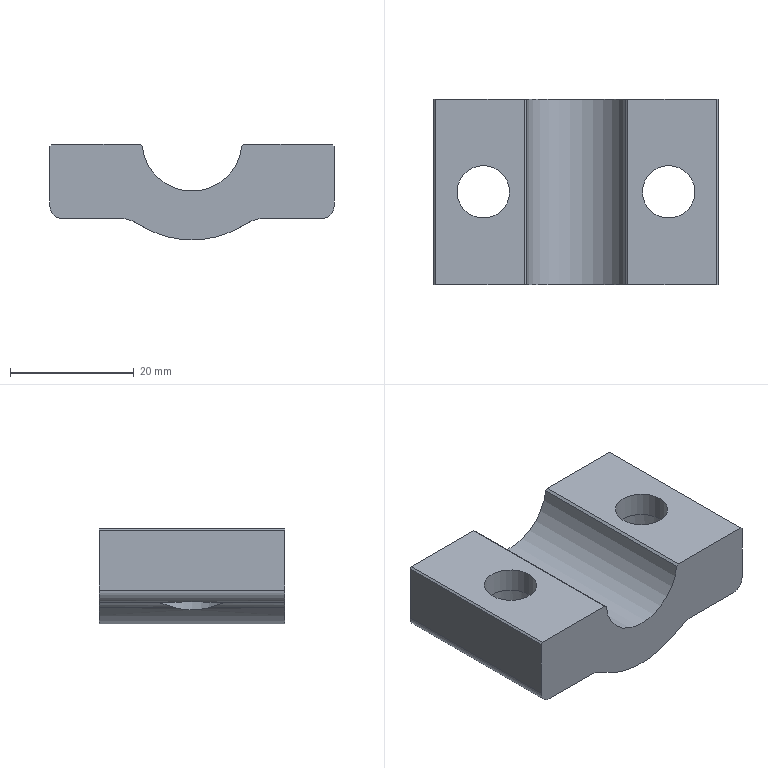NC program | NX | posted with a generic post | part box 46 x 30 x 15.5 mm
Whole program:
N10 G17 G21 G94 G90
(2D点孔 , TOOL : D10点钻)
N12 T04 M6
N14 G54
N16 G17 G0 G90 X-15. Y0. B0. C0. S2000 M3
N18 G43 Z30. H4
N20 G94 G81 G98 Z-5. F200. R-1.5
N22 X15.
N24 G80
N26 G0 X15. Y0. Z30.
N28 M5
(2D点孔_COPY , TOOL : Z8.5)
N30 T05 M6
N32 G54
N34 G17 G0 G90 X-15. Y0. B0. C0. S1600 M3
N36 G43 Z30. H5
N38 G94 G83 G98 Z-18.5 F150. Q2. R-1.5
N40 X15.
N42 G80
N44 G0 X15. Y0. Z30.
N46 M5
(孔铣螺旋 , TOOL : D10开粗)
N48 T02 M6
N50 G54
N52 G17 G0 G90 X-15. Y0. B0. C0. S3000 M3
N54 G43 Z30. H2
N56 Z-1.791
N58 G94 G3 X-15.825 Y0.825 R0.825 F800.
N60 X-16.65 Y0. R0.825
N62 X-16.65 Y0. Z-2.591 I1.65 J0.
N64 X-16.65 Y0. Z-3.391 I1.65 J0.
N66 X-16.65 Y0. Z-4.191 I1.65 J0.
N68 X-16.65 Y0. Z-4.991 I1.65 J0.
N70 X-16.65 Y0. Z-5.791 I1.65 J0.
N72 X-16.65 Y0. Z-6.591 I1.65 J0.
N74 X-16.65 Y0. Z-7.391 I1.65 J0.
N76 X-16.65 Y0. Z-8.191 I1.65 J0.
N78 X-16.65 Y0. Z-8.991 I1.65 J0.
N80 X-16.65 Y0. Z-9.791 I1.65 J0.
N82 X-16.65 Y0. Z-10.591 I1.65 J0.
N84 X-16.65 Y0. Z-11.391 I1.65 J0.
N86 X-16.081 Y-1.246 Z-11.5 R1.65
N88 X-13.754 Y-1.081 R1.65
N90 X-16.081 Y-1.246 R-1.65
N92 X-14.917 Y-1.164 R0.825
N94 X-15. Y0. R0.825
N96 G0 Z15.855
N98 X15.
N100 Z-1.791
N102 G3 X14.175 Y0.825 R0.825
N104 X13.35 Y0. R0.825
N106 X13.35 Y0. Z-2.591 I1.65 J0.
N108 X13.35 Y0. Z-3.391 I1.65 J0.
N110 X13.35 Y0. Z-4.191 I1.65 J0.
N112 X13.35 Y0. Z-4.991 I1.65 J0.
N114 X13.35 Y0. Z-5.791 I1.65 J0.
N116 X13.35 Y0. Z-6.591 I1.65 J0.
N118 X13.35 Y0. Z-7.391 I1.65 J0.
N120 X13.35 Y0. Z-8.191 I1.65 J0.
N122 X13.35 Y0. Z-8.991 I1.65 J0.
N124 X13.35 Y0. Z-9.791 I1.65 J0.
N126 X13.35 Y0. Z-10.591 I1.65 J0.
N128 X13.35 Y0. Z-11.391 I1.65 J0.
N130 X13.919 Y-1.246 Z-11.5 R1.65
N132 X16.246 Y-1.081 R1.65
N134 X13.919 Y-1.246 R-1.65
N136 X15.083 Y-1.164 R0.825
N138 X15. Y0. R0.825
N140 G0 Z30.
N142 M5
(孔铣螺旋_COPY , TOOL : D10精光)
N144 T03 M6
N146 G54
N148 G17 G0 G90 X-15. Y0. B0. C0. S3000 M3
N150 G43 Z30. H3
N152 Z-11.5
N154 G94 G3 X-15.875 Y0.875 R0.875 F300.
N156 X-16.75 Y0. R0.875
N158 X-15. Y-1.75 R1.75
N160 X-16.75 Y0. R-1.75
N162 X-15.875 Y-0.875 R0.875
N164 X-15. Y0. R0.875
N166 G0 Z16.355
N168 X15.
N170 Z-11.5
N172 G3 X14.125 Y0.875 R0.875
N174 X13.25 Y0. R0.875
N176 X15. Y-1.75 R1.75
N178 X13.25 Y0. R-1.75
N180 X14.125 Y-0.875 R0.875
N182 X15. Y0. R0.875
N184 G0 Z30.
N186 M5
N188 M2